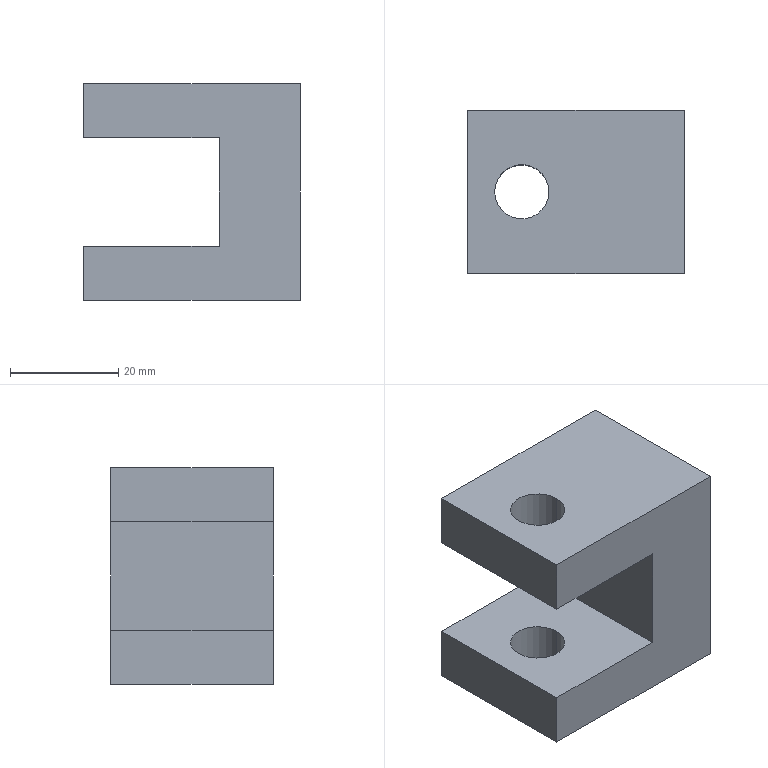Part | SolidWorks | features Extrusion 1, ICE 1 | 1 solid | 14 faces | box 40 x 30 x 40 mm | volume 31429 mm3 | plane 10 | cylinder 4 | commonest cylinder face diameters 10 x4
STEP:
#1=CARTESIAN_POINT('',(-5.,15.,-10.));
#2=VERTEX_POINT('',#1);
#3=CARTESIAN_POINT('',(-15.,15.,-10.));
#4=VERTEX_POINT('',#3);
#5=CARTESIAN_POINT('',(-10.,15.,-10.));
#6=DIRECTION('',(0.,0.,-1.));
#7=DIRECTION('',(-1.,0.,0.));
#8=AXIS2_PLACEMENT_3D('',#5,#6,#7);
#9=CIRCLE('',#8,5.);
#10=EDGE_CURVE('',#2,#4,#9,.T.);
#11=ORIENTED_EDGE('',*,*,#10,.F.);
#12=CARTESIAN_POINT('',(-5.,15.,-20.));
#13=VERTEX_POINT('',#12);
#14=CARTESIAN_POINT('',(-5.,15.,20.));
#15=DIRECTION('',(0.,0.,-1.));
#16=VECTOR('',#15,1000.);
#17=LINE('',#14,#16);
#18=EDGE_CURVE('',#2,#13,#17,.T.);
#19=ORIENTED_EDGE('',*,*,#18,.T.);
#20=CARTESIAN_POINT('',(-15.,15.,-20.));
#21=VERTEX_POINT('',#20);
#22=CARTESIAN_POINT('',(-10.,15.,-20.));
#23=DIRECTION('',(0.,0.,-1.));
#24=DIRECTION('',(-1.,0.,0.));
#25=AXIS2_PLACEMENT_3D('',#22,#23,#24);
#26=CIRCLE('',#25,5.);
#27=EDGE_CURVE('',#13,#21,#26,.T.);
#28=ORIENTED_EDGE('',*,*,#27,.T.);
#29=CARTESIAN_POINT('',(-15.,15.,20.));
#30=DIRECTION('',(0.,0.,-1.));
#31=VECTOR('',#30,1000.);
#32=LINE('',#29,#31);
#33=EDGE_CURVE('',#4,#21,#32,.T.);
#34=ORIENTED_EDGE('',*,*,#33,.F.);
#35=EDGE_LOOP('',(#11,#19,#28,#34));
#36=FACE_OUTER_BOUND('',#35,.T.);
#37=CARTESIAN_POINT('',(-10.,15.,20.));
#38=DIRECTION('',(0.,0.,-1.));
#39=DIRECTION('',(-1.,0.,0.));
#40=AXIS2_PLACEMENT_3D('',#37,#38,#39);
#41=CYLINDRICAL_SURFACE('',#40,5.);
#42=ADVANCED_FACE('',(#36),#41,.F.);
#43=CARTESIAN_POINT('',(-5.,15.,20.));
#44=VERTEX_POINT('',#43);
#45=CARTESIAN_POINT('',(-15.,15.,20.));
#46=VERTEX_POINT('',#45);
#47=CARTESIAN_POINT('',(-10.,15.,20.));
#48=DIRECTION('',(0.,0.,-1.));
#49=DIRECTION('',(-1.,0.,0.));
#50=AXIS2_PLACEMENT_3D('',#47,#48,#49);
#51=CIRCLE('',#50,5.);
#52=EDGE_CURVE('',#44,#46,#51,.T.);
#53=ORIENTED_EDGE('',*,*,#52,.F.);
#54=CARTESIAN_POINT('',(-5.,15.,10.));
#55=VERTEX_POINT('',#54);
#56=CARTESIAN_POINT('',(-5.,15.,20.));
#57=DIRECTION('',(0.,0.,-1.));
#58=VECTOR('',#57,1000.);
#59=LINE('',#56,#58);
#60=EDGE_CURVE('',#44,#55,#59,.T.);
#61=ORIENTED_EDGE('',*,*,#60,.T.);
#62=CARTESIAN_POINT('',(-15.,15.,10.));
#63=VERTEX_POINT('',#62);
#64=CARTESIAN_POINT('',(-10.,15.,10.));
#65=DIRECTION('',(0.,0.,1.));
#66=DIRECTION('',(1.,0.,0.));
#67=AXIS2_PLACEMENT_3D('',#64,#65,#66);
#68=CIRCLE('',#67,5.);
#69=EDGE_CURVE('',#63,#55,#68,.T.);
#70=ORIENTED_EDGE('',*,*,#69,.F.);
#71=CARTESIAN_POINT('',(-15.,15.,20.));
#72=DIRECTION('',(0.,0.,-1.));
#73=VECTOR('',#72,1000.);
#74=LINE('',#71,#73);
#75=EDGE_CURVE('',#46,#63,#74,.T.);
#76=ORIENTED_EDGE('',*,*,#75,.F.);
#77=EDGE_LOOP('',(#53,#61,#70,#76));
#78=FACE_OUTER_BOUND('',#77,.T.);
#79=CARTESIAN_POINT('',(-10.,15.,20.));
#80=DIRECTION('',(0.,0.,-1.));
#81=DIRECTION('',(-1.,0.,0.));
#82=AXIS2_PLACEMENT_3D('',#79,#80,#81);
#83=CYLINDRICAL_SURFACE('',#82,5.);
#84=ADVANCED_FACE('',(#78),#83,.F.);
#85=CARTESIAN_POINT('',(20.,0.,20.));
#86=VERTEX_POINT('',#85);
#87=CARTESIAN_POINT('',(20.,0.,-20.));
#88=VERTEX_POINT('',#87);
#89=CARTESIAN_POINT('',(20.,0.,20.));
#90=DIRECTION('',(0.,0.,-1.));
#91=VECTOR('',#90,1000.);
#92=LINE('',#89,#91);
#93=EDGE_CURVE('',#86,#88,#92,.T.);
#94=ORIENTED_EDGE('',*,*,#93,.T.);
#95=CARTESIAN_POINT('',(20.,30.,-20.));
#96=VERTEX_POINT('',#95);
#97=CARTESIAN_POINT('',(20.,30.,-20.));
#98=DIRECTION('',(0.,-1.,0.));
#99=VECTOR('',#98,1000.);
#100=LINE('',#97,#99);
#101=EDGE_CURVE('',#96,#88,#100,.T.);
#102=ORIENTED_EDGE('',*,*,#101,.F.);
#103=CARTESIAN_POINT('',(20.,30.,20.));
#104=VERTEX_POINT('',#103);
#105=CARTESIAN_POINT('',(20.,30.,20.));
#106=DIRECTION('',(0.,0.,-1.));
#107=VECTOR('',#106,1000.);
#108=LINE('',#105,#107);
#109=EDGE_CURVE('',#104,#96,#108,.T.);
#110=ORIENTED_EDGE('',*,*,#109,.F.);
#111=CARTESIAN_POINT('',(20.,30.,20.));
#112=DIRECTION('',(0.,-1.,0.));
#113=VECTOR('',#112,1000.);
#114=LINE('',#111,#113);
#115=EDGE_CURVE('',#104,#86,#114,.T.);
#116=ORIENTED_EDGE('',*,*,#115,.T.);
#117=EDGE_LOOP('',(#94,#102,#110,#116));
#118=FACE_OUTER_BOUND('',#117,.T.);
#119=CARTESIAN_POINT('',(20.,30.,20.));
#120=DIRECTION('',(-1.,0.,0.));
#121=DIRECTION('',(0.,0.,1.));
#122=AXIS2_PLACEMENT_3D('',#119,#120,#121);
#123=PLANE('',#122);
#124=ADVANCED_FACE('',(#118),#123,.F.);
#125=CARTESIAN_POINT('',(-10.,15.,-20.));
#126=DIRECTION('',(0.,0.,-1.));
#127=DIRECTION('',(-1.,0.,0.));
#128=AXIS2_PLACEMENT_3D('',#125,#126,#127);
#129=CIRCLE('',#128,5.);
#130=EDGE_CURVE('',#21,#13,#129,.T.);
#131=ORIENTED_EDGE('',*,*,#130,.F.);
#132=ORIENTED_EDGE('',*,*,#27,.F.);
#133=EDGE_LOOP('',(#131,#132));
#134=FACE_BOUND('',#133,.T.);
#135=CARTESIAN_POINT('',(-20.,0.,-20.));
#136=VERTEX_POINT('',#135);
#137=CARTESIAN_POINT('',(-20.,0.,-20.));
#138=DIRECTION('',(-1.,0.,0.));
#139=VECTOR('',#138,1000.);
#140=LINE('',#137,#139);
#141=EDGE_CURVE('',#88,#136,#140,.T.);
#142=ORIENTED_EDGE('',*,*,#141,.T.);
#143=CARTESIAN_POINT('',(-20.,30.,-20.));
#144=VERTEX_POINT('',#143);
#145=CARTESIAN_POINT('',(-20.,30.,-20.));
#146=DIRECTION('',(0.,-1.,0.));
#147=VECTOR('',#146,1000.);
#148=LINE('',#145,#147);
#149=EDGE_CURVE('',#144,#136,#148,.T.);
#150=ORIENTED_EDGE('',*,*,#149,.F.);
#151=CARTESIAN_POINT('',(-20.,30.,-20.));
#152=DIRECTION('',(-1.,0.,0.));
#153=VECTOR('',#152,1000.);
#154=LINE('',#151,#153);
#155=EDGE_CURVE('',#96,#144,#154,.T.);
#156=ORIENTED_EDGE('',*,*,#155,.F.);
#157=ORIENTED_EDGE('',*,*,#101,.T.);
#158=EDGE_LOOP('',(#142,#150,#156,#157));
#159=FACE_OUTER_BOUND('',#158,.T.);
#160=CARTESIAN_POINT('',(-20.,30.,-20.));
#161=DIRECTION('',(0.,0.,1.));
#162=DIRECTION('',(1.,0.,0.));
#163=AXIS2_PLACEMENT_3D('',#160,#161,#162);
#164=PLANE('',#163);
#165=ADVANCED_FACE('',(#134,#159),#164,.F.);
#166=CARTESIAN_POINT('',(-20.,0.,-10.));
#167=VERTEX_POINT('',#166);
#168=CARTESIAN_POINT('',(-20.,0.,-10.));
#169=DIRECTION('',(0.,0.,1.));
#170=VECTOR('',#169,1000.);
#171=LINE('',#168,#170);
#172=EDGE_CURVE('',#136,#167,#171,.T.);
#173=ORIENTED_EDGE('',*,*,#172,.T.);
#174=CARTESIAN_POINT('',(-20.,30.,-10.));
#175=VERTEX_POINT('',#174);
#176=CARTESIAN_POINT('',(-20.,30.,-10.));
#177=DIRECTION('',(0.,-1.,0.));
#178=VECTOR('',#177,1000.);
#179=LINE('',#176,#178);
#180=EDGE_CURVE('',#175,#167,#179,.T.);
#181=ORIENTED_EDGE('',*,*,#180,.F.);
#182=CARTESIAN_POINT('',(-20.,30.,-10.));
#183=DIRECTION('',(0.,0.,1.));
#184=VECTOR('',#183,1000.);
#185=LINE('',#182,#184);
#186=EDGE_CURVE('',#144,#175,#185,.T.);
#187=ORIENTED_EDGE('',*,*,#186,.F.);
#188=ORIENTED_EDGE('',*,*,#149,.T.);
#189=EDGE_LOOP('',(#173,#181,#187,#188));
#190=FACE_OUTER_BOUND('',#189,.T.);
#191=CARTESIAN_POINT('',(-20.,30.,-10.));
#192=DIRECTION('',(1.,0.,0.));
#193=DIRECTION('',(0.,0.,-1.));
#194=AXIS2_PLACEMENT_3D('',#191,#192,#193);
#195=PLANE('',#194);
#196=ADVANCED_FACE('',(#190),#195,.F.);
#197=CARTESIAN_POINT('',(-10.,15.,-10.));
#198=DIRECTION('',(0.,0.,-1.));
#199=DIRECTION('',(-1.,0.,0.));
#200=AXIS2_PLACEMENT_3D('',#197,#198,#199);
#201=CIRCLE('',#200,5.);
#202=EDGE_CURVE('',#4,#2,#201,.T.);
#203=ORIENTED_EDGE('',*,*,#202,.T.);
#204=ORIENTED_EDGE('',*,*,#10,.T.);
#205=EDGE_LOOP('',(#203,#204));
#206=FACE_BOUND('',#205,.T.);
#207=CARTESIAN_POINT('',(5.,0.,-10.));
#208=VERTEX_POINT('',#207);
#209=CARTESIAN_POINT('',(-20.,0.,-10.));
#210=DIRECTION('',(1.,0.,0.));
#211=VECTOR('',#210,1000.);
#212=LINE('',#209,#211);
#213=EDGE_CURVE('',#167,#208,#212,.T.);
#214=ORIENTED_EDGE('',*,*,#213,.T.);
#215=CARTESIAN_POINT('',(5.,30.,-10.));
#216=VERTEX_POINT('',#215);
#217=CARTESIAN_POINT('',(5.,30.,-10.));
#218=DIRECTION('',(0.,-1.,0.));
#219=VECTOR('',#218,1000.);
#220=LINE('',#217,#219);
#221=EDGE_CURVE('',#216,#208,#220,.T.);
#222=ORIENTED_EDGE('',*,*,#221,.F.);
#223=CARTESIAN_POINT('',(-20.,30.,-10.));
#224=DIRECTION('',(1.,0.,0.));
#225=VECTOR('',#224,1000.);
#226=LINE('',#223,#225);
#227=EDGE_CURVE('',#175,#216,#226,.T.);
#228=ORIENTED_EDGE('',*,*,#227,.F.);
#229=ORIENTED_EDGE('',*,*,#180,.T.);
#230=EDGE_LOOP('',(#214,#222,#228,#229));
#231=FACE_OUTER_BOUND('',#230,.T.);
#232=CARTESIAN_POINT('',(-20.,30.,-10.));
#233=DIRECTION('',(0.,0.,-1.));
#234=DIRECTION('',(-1.,0.,0.));
#235=AXIS2_PLACEMENT_3D('',#232,#233,#234);
#236=PLANE('',#235);
#237=ADVANCED_FACE('',(#206,#231),#236,.F.);
#238=CARTESIAN_POINT('',(5.,0.,10.));
#239=VERTEX_POINT('',#238);
#240=CARTESIAN_POINT('',(5.,0.,-10.));
#241=DIRECTION('',(0.,0.,1.));
#242=VECTOR('',#241,1000.);
#243=LINE('',#240,#242);
#244=EDGE_CURVE('',#208,#239,#243,.T.);
#245=ORIENTED_EDGE('',*,*,#244,.T.);
#246=CARTESIAN_POINT('',(5.,30.,10.));
#247=VERTEX_POINT('',#246);
#248=CARTESIAN_POINT('',(5.,30.,10.));
#249=DIRECTION('',(0.,-1.,0.));
#250=VECTOR('',#249,1000.);
#251=LINE('',#248,#250);
#252=EDGE_CURVE('',#247,#239,#251,.T.);
#253=ORIENTED_EDGE('',*,*,#252,.F.);
#254=CARTESIAN_POINT('',(5.,30.,-10.));
#255=DIRECTION('',(0.,0.,1.));
#256=VECTOR('',#255,1000.);
#257=LINE('',#254,#256);
#258=EDGE_CURVE('',#216,#247,#257,.T.);
#259=ORIENTED_EDGE('',*,*,#258,.F.);
#260=ORIENTED_EDGE('',*,*,#221,.T.);
#261=EDGE_LOOP('',(#245,#253,#259,#260));
#262=FACE_OUTER_BOUND('',#261,.T.);
#263=CARTESIAN_POINT('',(5.,30.,-10.));
#264=DIRECTION('',(1.,0.,0.));
#265=DIRECTION('',(0.,0.,-1.));
#266=AXIS2_PLACEMENT_3D('',#263,#264,#265);
#267=PLANE('',#266);
#268=ADVANCED_FACE('',(#262),#267,.F.);
#269=ORIENTED_EDGE('',*,*,#69,.T.);
#270=CARTESIAN_POINT('',(-10.,15.,10.));
#271=DIRECTION('',(0.,0.,1.));
#272=DIRECTION('',(1.,0.,0.));
#273=AXIS2_PLACEMENT_3D('',#270,#271,#272);
#274=CIRCLE('',#273,5.);
#275=EDGE_CURVE('',#55,#63,#274,.T.);
#276=ORIENTED_EDGE('',*,*,#275,.T.);
#277=EDGE_LOOP('',(#269,#276));
#278=FACE_BOUND('',#277,.T.);
#279=CARTESIAN_POINT('',(-20.,0.,10.));
#280=VERTEX_POINT('',#279);
#281=CARTESIAN_POINT('',(-20.,0.,10.));
#282=DIRECTION('',(-1.,0.,0.));
#283=VECTOR('',#282,1000.);
#284=LINE('',#281,#283);
#285=EDGE_CURVE('',#239,#280,#284,.T.);
#286=ORIENTED_EDGE('',*,*,#285,.T.);
#287=CARTESIAN_POINT('',(-20.,30.,10.));
#288=VERTEX_POINT('',#287);
#289=CARTESIAN_POINT('',(-20.,30.,10.));
#290=DIRECTION('',(0.,-1.,0.));
#291=VECTOR('',#290,1000.);
#292=LINE('',#289,#291);
#293=EDGE_CURVE('',#288,#280,#292,.T.);
#294=ORIENTED_EDGE('',*,*,#293,.F.);
#295=CARTESIAN_POINT('',(-20.,30.,10.));
#296=DIRECTION('',(-1.,0.,0.));
#297=VECTOR('',#296,1000.);
#298=LINE('',#295,#297);
#299=EDGE_CURVE('',#247,#288,#298,.T.);
#300=ORIENTED_EDGE('',*,*,#299,.F.);
#301=ORIENTED_EDGE('',*,*,#252,.T.);
#302=EDGE_LOOP('',(#286,#294,#300,#301));
#303=FACE_OUTER_BOUND('',#302,.T.);
#304=CARTESIAN_POINT('',(-20.,30.,10.));
#305=DIRECTION('',(0.,0.,1.));
#306=DIRECTION('',(1.,0.,0.));
#307=AXIS2_PLACEMENT_3D('',#304,#305,#306);
#308=PLANE('',#307);
#309=ADVANCED_FACE('',(#278,#303),#308,.F.);
#310=CARTESIAN_POINT('',(-20.,0.,20.));
#311=VERTEX_POINT('',#310);
#312=CARTESIAN_POINT('',(-20.,0.,20.));
#313=DIRECTION('',(0.,0.,1.));
#314=VECTOR('',#313,1000.);
#315=LINE('',#312,#314);
#316=EDGE_CURVE('',#280,#311,#315,.T.);
#317=ORIENTED_EDGE('',*,*,#316,.T.);
#318=CARTESIAN_POINT('',(-20.,30.,20.));
#319=VERTEX_POINT('',#318);
#320=CARTESIAN_POINT('',(-20.,30.,20.));
#321=DIRECTION('',(0.,-1.,0.));
#322=VECTOR('',#321,1000.);
#323=LINE('',#320,#322);
#324=EDGE_CURVE('',#319,#311,#323,.T.);
#325=ORIENTED_EDGE('',*,*,#324,.F.);
#326=CARTESIAN_POINT('',(-20.,30.,20.));
#327=DIRECTION('',(0.,0.,1.));
#328=VECTOR('',#327,1000.);
#329=LINE('',#326,#328);
#330=EDGE_CURVE('',#288,#319,#329,.T.);
#331=ORIENTED_EDGE('',*,*,#330,.F.);
#332=ORIENTED_EDGE('',*,*,#293,.T.);
#333=EDGE_LOOP('',(#317,#325,#331,#332));
#334=FACE_OUTER_BOUND('',#333,.T.);
#335=CARTESIAN_POINT('',(-20.,30.,20.));
#336=DIRECTION('',(1.,0.,0.));
#337=DIRECTION('',(0.,0.,-1.));
#338=AXIS2_PLACEMENT_3D('',#335,#336,#337);
#339=PLANE('',#338);
#340=ADVANCED_FACE('',(#334),#339,.F.);
#341=CARTESIAN_POINT('',(-10.,15.,20.));
#342=DIRECTION('',(0.,0.,-1.));
#343=DIRECTION('',(-1.,0.,0.));
#344=AXIS2_PLACEMENT_3D('',#341,#342,#343);
#345=CIRCLE('',#344,5.);
#346=EDGE_CURVE('',#46,#44,#345,.T.);
#347=ORIENTED_EDGE('',*,*,#346,.T.);
#348=ORIENTED_EDGE('',*,*,#52,.T.);
#349=EDGE_LOOP('',(#347,#348));
#350=FACE_BOUND('',#349,.T.);
#351=CARTESIAN_POINT('',(-20.,0.,20.));
#352=DIRECTION('',(1.,0.,0.));
#353=VECTOR('',#352,1000.);
#354=LINE('',#351,#353);
#355=EDGE_CURVE('',#311,#86,#354,.T.);
#356=ORIENTED_EDGE('',*,*,#355,.T.);
#357=ORIENTED_EDGE('',*,*,#115,.F.);
#358=CARTESIAN_POINT('',(-20.,30.,20.));
#359=DIRECTION('',(1.,0.,0.));
#360=VECTOR('',#359,1000.);
#361=LINE('',#358,#360);
#362=EDGE_CURVE('',#319,#104,#361,.T.);
#363=ORIENTED_EDGE('',*,*,#362,.F.);
#364=ORIENTED_EDGE('',*,*,#324,.T.);
#365=EDGE_LOOP('',(#356,#357,#363,#364));
#366=FACE_OUTER_BOUND('',#365,.T.);
#367=CARTESIAN_POINT('',(-20.,30.,20.));
#368=DIRECTION('',(0.,0.,-1.));
#369=DIRECTION('',(-1.,0.,0.));
#370=AXIS2_PLACEMENT_3D('',#367,#368,#369);
#371=PLANE('',#370);
#372=ADVANCED_FACE('',(#350,#366),#371,.F.);
#373=ORIENTED_EDGE('',*,*,#109,.T.);
#374=ORIENTED_EDGE('',*,*,#155,.T.);
#375=ORIENTED_EDGE('',*,*,#186,.T.);
#376=ORIENTED_EDGE('',*,*,#227,.T.);
#377=ORIENTED_EDGE('',*,*,#258,.T.);
#378=ORIENTED_EDGE('',*,*,#299,.T.);
#379=ORIENTED_EDGE('',*,*,#330,.T.);
#380=ORIENTED_EDGE('',*,*,#362,.T.);
#381=EDGE_LOOP('',(#373,#374,#375,#376,#377,#378,#379,#380));
#382=FACE_OUTER_BOUND('',#381,.T.);
#383=CARTESIAN_POINT('',(0.,30.,0.));
#384=DIRECTION('',(0.,-1.,0.));
#385=DIRECTION('',(0.,0.,-1.));
#386=AXIS2_PLACEMENT_3D('',#383,#384,#385);
#387=PLANE('',#386);
#388=ADVANCED_FACE('',(#382),#387,.F.);
#389=ORIENTED_EDGE('',*,*,#93,.F.);
#390=ORIENTED_EDGE('',*,*,#355,.F.);
#391=ORIENTED_EDGE('',*,*,#316,.F.);
#392=ORIENTED_EDGE('',*,*,#285,.F.);
#393=ORIENTED_EDGE('',*,*,#244,.F.);
#394=ORIENTED_EDGE('',*,*,#213,.F.);
#395=ORIENTED_EDGE('',*,*,#172,.F.);
#396=ORIENTED_EDGE('',*,*,#141,.F.);
#397=EDGE_LOOP('',(#389,#390,#391,#392,#393,#394,#395,#396));
#398=FACE_OUTER_BOUND('',#397,.T.);
#399=CARTESIAN_POINT('',(0.,0.,0.));
#400=DIRECTION('',(0.,-1.,0.));
#401=DIRECTION('',(0.,0.,-1.));
#402=AXIS2_PLACEMENT_3D('',#399,#400,#401);
#403=PLANE('',#402);
#404=ADVANCED_FACE('',(#398),#403,.T.);
#405=ORIENTED_EDGE('',*,*,#60,.F.);
#406=ORIENTED_EDGE('',*,*,#346,.F.);
#407=ORIENTED_EDGE('',*,*,#75,.T.);
#408=ORIENTED_EDGE('',*,*,#275,.F.);
#409=EDGE_LOOP('',(#405,#406,#407,#408));
#410=FACE_OUTER_BOUND('',#409,.T.);
#411=CARTESIAN_POINT('',(-10.,15.,20.));
#412=DIRECTION('',(0.,0.,-1.));
#413=DIRECTION('',(-1.,0.,0.));
#414=AXIS2_PLACEMENT_3D('',#411,#412,#413);
#415=CYLINDRICAL_SURFACE('',#414,5.);
#416=ADVANCED_FACE('',(#410),#415,.F.);
#417=ORIENTED_EDGE('',*,*,#18,.F.);
#418=ORIENTED_EDGE('',*,*,#202,.F.);
#419=ORIENTED_EDGE('',*,*,#33,.T.);
#420=ORIENTED_EDGE('',*,*,#130,.T.);
#421=EDGE_LOOP('',(#417,#418,#419,#420));
#422=FACE_OUTER_BOUND('',#421,.T.);
#423=CARTESIAN_POINT('',(-10.,15.,20.));
#424=DIRECTION('',(0.,0.,-1.));
#425=DIRECTION('',(-1.,0.,0.));
#426=AXIS2_PLACEMENT_3D('',#423,#424,#425);
#427=CYLINDRICAL_SURFACE('',#426,5.);
#428=ADVANCED_FACE('',(#422),#427,.F.);
#429=CLOSED_SHELL('',(#42,#84,#124,#165,#196,#237,#268,#309,#340,#372,#388,#404,#416,#428));
#430=MANIFOLD_SOLID_BREP('',#429);
#431=CARTESIAN_POINT('',(0.,0.,0.));
#432=DIRECTION('',(0.,0.,1.));
#433=DIRECTION('',(1.,0.,0.));
#434=AXIS2_PLACEMENT_3D('',#431,#432,#433);
#435=(LENGTH_UNIT()NAMED_UNIT(*)SI_UNIT(.MILLI.,.METRE.));
#436=UNCERTAINTY_MEASURE_WITH_UNIT(LENGTH_MEASURE(0.00001),#435,'','');
#437=(NAMED_UNIT(*)PLANE_ANGLE_UNIT()SI_UNIT($,.RADIAN.));
#438=(NAMED_UNIT(*)SI_UNIT($,.STERADIAN.)SOLID_ANGLE_UNIT());
#439=(GEOMETRIC_REPRESENTATION_CONTEXT(3)GLOBAL_UNCERTAINTY_ASSIGNED_CONTEXT((#436))GLOBAL_UNIT_ASSIGNED_CONTEXT((#435,#437,#438))REPRESENTATION_CONTEXT('',''));
#440=ADVANCED_BREP_SHAPE_REPRESENTATION('',(#430,#434),#439);